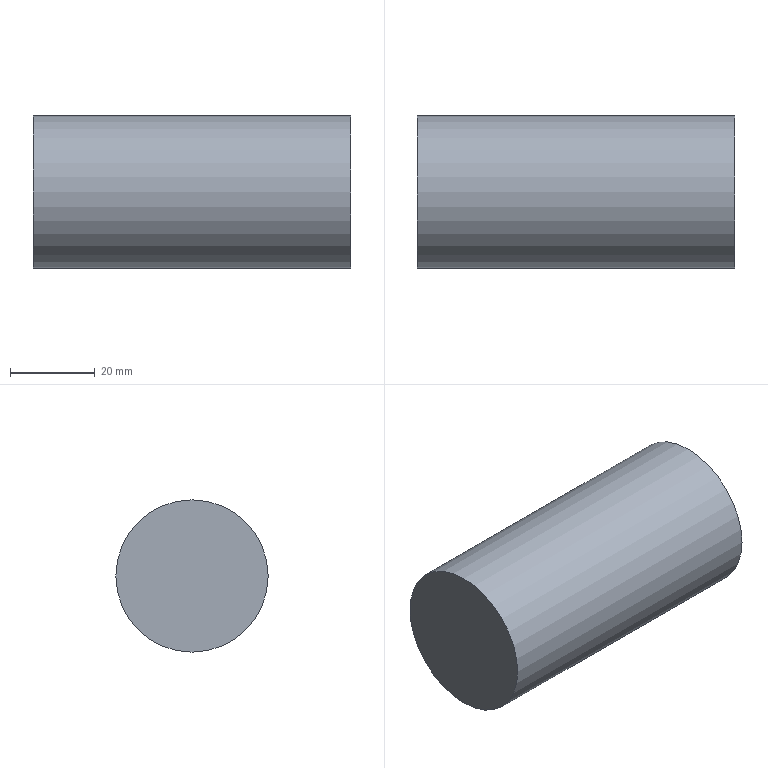Part | NX | features solid 2 | 1 solid | 3 faces | box 75 x 36 x 36 mm | volume 76341 mm3 | plane 2 | cylinder 1 | commonest cylinder face diameters 36 x1
STEP:
#1=CARTESIAN_POINT('',(-664.,162.,-295.));
#2=VERTEX_POINT('',#1);
#3=CARTESIAN_POINT('',(-664.,180.,-295.));
#4=DIRECTION('',(-1.,0.,0.));
#5=DIRECTION('',(0.,-1.,0.));
#6=AXIS2_PLACEMENT_3D('',#3,#4,#5);
#7=CIRCLE('',#6,18.);
#8=EDGE_CURVE('',#2,#2,#7,.T.);
#9=ORIENTED_EDGE('',*,*,#8,.T.);
#10=EDGE_LOOP('',(#9));
#11=FACE_BOUND('',#10,.T.);
#12=CARTESIAN_POINT('',(-664.,180.,-295.));
#13=DIRECTION('',(-1.,0.,0.));
#14=DIRECTION('',(0.,-1.,0.));
#15=AXIS2_PLACEMENT_3D('',#12,#13,#14);
#16=PLANE('',#15);
#17=ADVANCED_FACE('',(#11),#16,.T.);
#18=CARTESIAN_POINT('',(-589.,180.,-277.));
#19=VERTEX_POINT('',#18);
#20=CARTESIAN_POINT('',(-589.,180.,-295.));
#21=DIRECTION('',(-1.,0.,0.));
#22=DIRECTION('',(0.,0.,1.));
#23=AXIS2_PLACEMENT_3D('',#20,#21,#22);
#24=CIRCLE('',#23,18.);
#25=EDGE_CURVE('',#19,#19,#24,.T.);
#26=ORIENTED_EDGE('',*,*,#25,.T.);
#27=EDGE_LOOP('',(#26));
#28=FACE_BOUND('',#27,.T.);
#29=ORIENTED_EDGE('',*,*,#8,.F.);
#30=EDGE_LOOP('',(#29));
#31=FACE_BOUND('',#30,.T.);
#32=CARTESIAN_POINT('',(-664.,180.,-295.));
#33=DIRECTION('',(1.,0.,0.));
#34=DIRECTION('',(0.,1.,0.));
#35=AXIS2_PLACEMENT_3D('',#32,#33,#34);
#36=CYLINDRICAL_SURFACE('',#35,18.);
#37=ADVANCED_FACE('',(#28,#31),#36,.T.);
#38=ORIENTED_EDGE('',*,*,#25,.F.);
#39=EDGE_LOOP('',(#38));
#40=FACE_BOUND('',#39,.T.);
#41=CARTESIAN_POINT('',(-589.,180.,-295.));
#42=DIRECTION('',(-1.,0.,0.));
#43=DIRECTION('',(0.,0.,-1.));
#44=AXIS2_PLACEMENT_3D('',#41,#42,#43);
#45=PLANE('',#44);
#46=ADVANCED_FACE('',(#40),#45,.F.);
#47=CLOSED_SHELL('',(#17,#37,#46));
#48=MANIFOLD_SOLID_BREP('',#47);
#49=(LENGTH_UNIT()NAMED_UNIT(*)SI_UNIT(.MILLI.,.METRE.));
#50=UNCERTAINTY_MEASURE_WITH_UNIT(LENGTH_MEASURE(0.00001),#49,'','');
#51=(NAMED_UNIT(*)PLANE_ANGLE_UNIT()SI_UNIT($,.RADIAN.));
#52=(NAMED_UNIT(*)SI_UNIT($,.STERADIAN.)SOLID_ANGLE_UNIT());
#53=(GEOMETRIC_REPRESENTATION_CONTEXT(3)GLOBAL_UNCERTAINTY_ASSIGNED_CONTEXT((#50))GLOBAL_UNIT_ASSIGNED_CONTEXT((#49,#51,#52))REPRESENTATION_CONTEXT('',''));
#54=ADVANCED_BREP_SHAPE_REPRESENTATION('',(#48),#53);